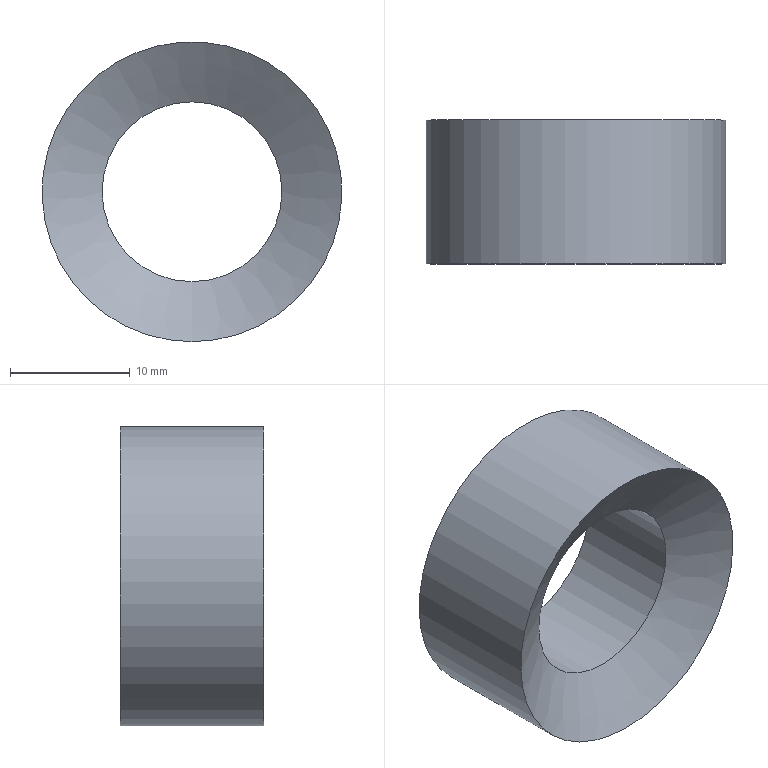Part | NX | features DATUM_CSYS 2, SKETCH 1, SWP104 1 | 1 solid | 4 faces | box 25 x 12 x 25 mm | volume 3354 mm3 | cylinder 2 | cone 1 | plane 1 | commonest cylinder face diameters 15 x1 25 x1
STEP:
#1=CARTESIAN_POINT('',(0.,0.,-7.5));
#2=VERTEX_POINT('',#1);
#3=CARTESIAN_POINT('',(0.,0.,0.));
#4=DIRECTION('',(0.,-1.,0.));
#5=DIRECTION('',(0.,0.,-1.));
#6=AXIS2_PLACEMENT_3D('',#3,#4,#5);
#7=CIRCLE('',#6,7.5);
#8=EDGE_CURVE('',#2,#2,#7,.T.);
#9=ORIENTED_EDGE('',*,*,#8,.F.);
#10=EDGE_LOOP('',(#9));
#11=FACE_BOUND('',#10,.T.);
#12=CARTESIAN_POINT('',(0.,-2.887,-12.5));
#13=VERTEX_POINT('',#12);
#14=CARTESIAN_POINT('',(0.,-2.887,0.));
#15=DIRECTION('',(0.,-1.,0.));
#16=DIRECTION('',(0.,0.,-1.));
#17=AXIS2_PLACEMENT_3D('',#14,#15,#16);
#18=CIRCLE('',#17,12.5);
#19=EDGE_CURVE('',#13,#13,#18,.T.);
#20=ORIENTED_EDGE('',*,*,#19,.T.);
#21=EDGE_LOOP('',(#20));
#22=FACE_BOUND('',#21,.T.);
#23=CARTESIAN_POINT('',(0.,-2.887,0.));
#24=DIRECTION('',(0.,-1.,0.));
#25=DIRECTION('',(0.,0.,-1.));
#26=AXIS2_PLACEMENT_3D('',#23,#24,#25);
#27=CONICAL_SURFACE('',#26,12.5,1.047);
#28=ADVANCED_FACE('',(#11,#22),#27,.F.);
#29=CARTESIAN_POINT('',(0.,9.113,-7.5));
#30=VERTEX_POINT('',#29);
#31=CARTESIAN_POINT('',(0.,9.113,0.));
#32=DIRECTION('',(0.,-1.,0.));
#33=DIRECTION('',(0.,0.,-1.));
#34=AXIS2_PLACEMENT_3D('',#31,#32,#33);
#35=CIRCLE('',#34,7.5);
#36=EDGE_CURVE('',#30,#30,#35,.T.);
#37=ORIENTED_EDGE('',*,*,#36,.F.);
#38=EDGE_LOOP('',(#37));
#39=FACE_BOUND('',#38,.T.);
#40=ORIENTED_EDGE('',*,*,#8,.T.);
#41=EDGE_LOOP('',(#40));
#42=FACE_BOUND('',#41,.T.);
#43=CARTESIAN_POINT('',(0.,0.,0.));
#44=DIRECTION('',(0.,-1.,0.));
#45=DIRECTION('',(0.,0.,-1.));
#46=AXIS2_PLACEMENT_3D('',#43,#44,#45);
#47=CYLINDRICAL_SURFACE('',#46,7.5);
#48=ADVANCED_FACE('',(#39,#42),#47,.F.);
#49=CARTESIAN_POINT('',(0.,9.113,-12.5));
#50=VERTEX_POINT('',#49);
#51=CARTESIAN_POINT('',(0.,9.113,0.));
#52=DIRECTION('',(0.,-1.,0.));
#53=DIRECTION('',(0.,0.,-1.));
#54=AXIS2_PLACEMENT_3D('',#51,#52,#53);
#55=CIRCLE('',#54,12.5);
#56=EDGE_CURVE('',#50,#50,#55,.T.);
#57=ORIENTED_EDGE('',*,*,#56,.F.);
#58=EDGE_LOOP('',(#57));
#59=FACE_BOUND('',#58,.T.);
#60=ORIENTED_EDGE('',*,*,#36,.T.);
#61=EDGE_LOOP('',(#60));
#62=FACE_BOUND('',#61,.T.);
#63=CARTESIAN_POINT('',(0.,9.113,7.5));
#64=DIRECTION('',(0.,-1.,0.));
#65=DIRECTION('',(0.,0.,-1.));
#66=AXIS2_PLACEMENT_3D('',#63,#64,#65);
#67=PLANE('',#66);
#68=ADVANCED_FACE('',(#59,#62),#67,.F.);
#69=ORIENTED_EDGE('',*,*,#19,.F.);
#70=EDGE_LOOP('',(#69));
#71=FACE_BOUND('',#70,.T.);
#72=ORIENTED_EDGE('',*,*,#56,.T.);
#73=EDGE_LOOP('',(#72));
#74=FACE_BOUND('',#73,.T.);
#75=CARTESIAN_POINT('',(0.,0.,0.));
#76=DIRECTION('',(0.,-1.,0.));
#77=DIRECTION('',(0.,0.,-1.));
#78=AXIS2_PLACEMENT_3D('',#75,#76,#77);
#79=CYLINDRICAL_SURFACE('',#78,12.5);
#80=ADVANCED_FACE('',(#71,#74),#79,.T.);
#81=CLOSED_SHELL('',(#28,#48,#68,#80));
#82=MANIFOLD_SOLID_BREP('',#81);
#83=(LENGTH_UNIT()NAMED_UNIT(*)SI_UNIT(.MILLI.,.METRE.));
#84=UNCERTAINTY_MEASURE_WITH_UNIT(LENGTH_MEASURE(0.00001),#83,'','');
#85=(NAMED_UNIT(*)PLANE_ANGLE_UNIT()SI_UNIT($,.RADIAN.));
#86=(NAMED_UNIT(*)SI_UNIT($,.STERADIAN.)SOLID_ANGLE_UNIT());
#87=(GEOMETRIC_REPRESENTATION_CONTEXT(3)GLOBAL_UNCERTAINTY_ASSIGNED_CONTEXT((#84))GLOBAL_UNIT_ASSIGNED_CONTEXT((#83,#85,#86))REPRESENTATION_CONTEXT('',''));
#88=ADVANCED_BREP_SHAPE_REPRESENTATION('',(#82),#87);